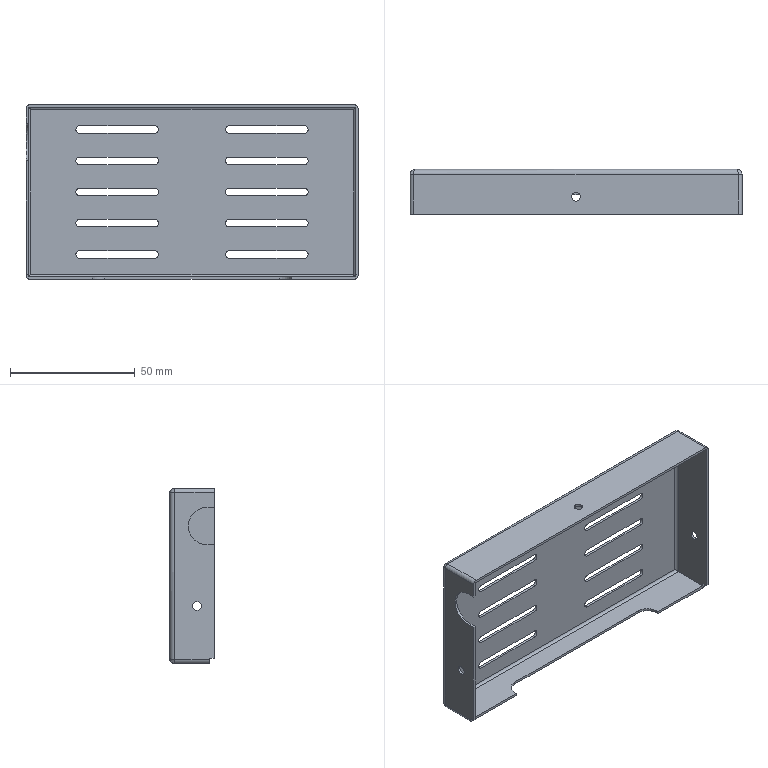Part | SolidWorks | features BaseBody 1 | 1 solid | 86 faces | box 133 x 18 x 70 mm | volume 13981 mm3 | cylinder 41 | plane 41 | spline 4 | commonest cylinder face diameters 3 x24 3.5 x6 2 x4 4 x4 10 x2 15 x1